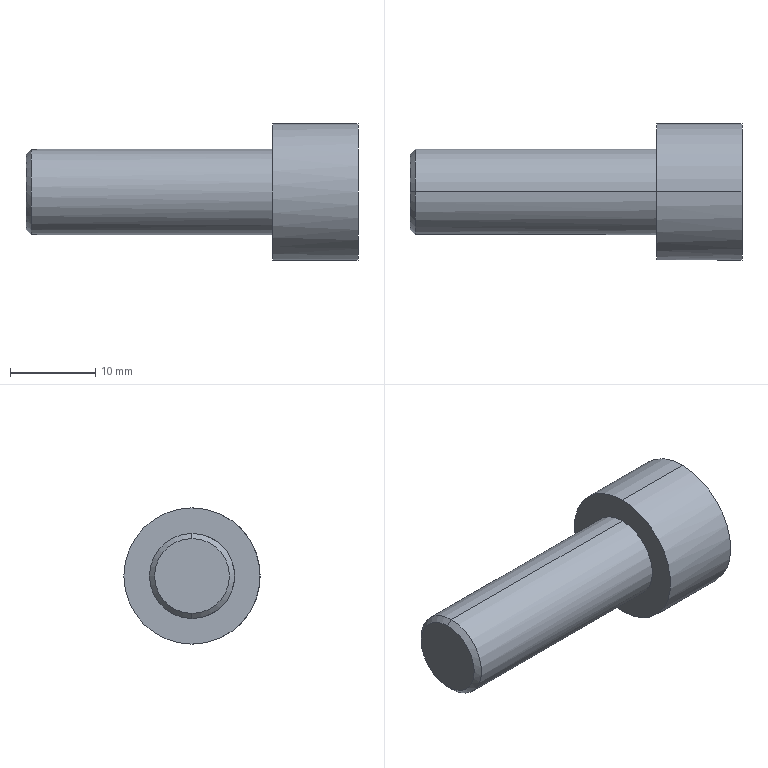Part | Creo | 1 solid | 16 faces | box 39 x 16 x 16 mm | volume 3917 mm3 | plane 10 | cylinder 4 | cone 2 | commonest cylinder face diameters 10 x2 16 x2
STEP:
#1=CARTESIAN_POINT('',(0.,0.,0.));
#2=DIRECTION('',(0.,0.,1.));
#3=DIRECTION('',(1.,0.,0.));
#4=AXIS2_PLACEMENT_3D('',#1,#2,#3);
#5=CARTESIAN_POINT('',(758.71,85.769,-129.619));
#6=VERTEX_POINT('',#5);
#7=CARTESIAN_POINT('',(758.71,90.769,-134.619));
#8=VERTEX_POINT('',#7);
#9=CARTESIAN_POINT('',(758.71,85.769,-134.619));
#10=DIRECTION('',(-1.,0.,0.));
#11=DIRECTION('',(0.,0.,1.));
#12=AXIS2_PLACEMENT_3D('',#9,#10,#11);
#13=CIRCLE('',#12,5.);
#14=EDGE_CURVE('',#6,#8,#13,.T.);
#15=ORIENTED_EDGE('',*,*,#14,.T.);
#16=CARTESIAN_POINT('',(758.71,85.769,-139.619));
#17=VERTEX_POINT('',#16);
#18=CARTESIAN_POINT('',(758.71,85.769,-134.619));
#19=DIRECTION('',(-1.,0.,0.));
#20=DIRECTION('',(0.,1.,0.));
#21=AXIS2_PLACEMENT_3D('',#18,#19,#20);
#22=CIRCLE('',#21,5.);
#23=EDGE_CURVE('',#8,#17,#22,.T.);
#24=ORIENTED_EDGE('',*,*,#23,.T.);
#25=CARTESIAN_POINT('',(787.101,85.769,-139.619));
#26=VERTEX_POINT('',#25);
#27=CARTESIAN_POINT('',(787.101,85.769,-139.619));
#28=DIRECTION('',(-1.,0.,0.));
#29=VECTOR('',#28,28.391);
#30=LINE('',#27,#29);
#31=EDGE_CURVE('',#26,#17,#30,.T.);
#32=ORIENTED_EDGE('',*,*,#31,.F.);
#33=CARTESIAN_POINT('',(787.101,90.769,-134.619));
#34=VERTEX_POINT('',#33);
#35=CARTESIAN_POINT('',(787.101,85.769,-134.619));
#36=DIRECTION('',(1.,0.,0.));
#37=DIRECTION('',(0.,0.,-1.));
#38=AXIS2_PLACEMENT_3D('',#35,#36,#37);
#39=CIRCLE('',#38,5.);
#40=EDGE_CURVE('',#26,#34,#39,.T.);
#41=ORIENTED_EDGE('',*,*,#40,.T.);
#42=CARTESIAN_POINT('',(787.101,85.769,-129.619));
#43=VERTEX_POINT('',#42);
#44=CARTESIAN_POINT('',(787.101,85.769,-134.619));
#45=DIRECTION('',(1.,0.,0.));
#46=DIRECTION('',(0.,1.,0.));
#47=AXIS2_PLACEMENT_3D('',#44,#45,#46);
#48=CIRCLE('',#47,5.);
#49=EDGE_CURVE('',#34,#43,#48,.T.);
#50=ORIENTED_EDGE('',*,*,#49,.T.);
#51=CARTESIAN_POINT('',(787.101,85.769,-129.619));
#52=DIRECTION('',(-1.,0.,0.));
#53=VECTOR('',#52,28.391);
#54=LINE('',#51,#53);
#55=EDGE_CURVE('',#43,#6,#54,.T.);
#56=ORIENTED_EDGE('',*,*,#55,.T.);
#57=EDGE_LOOP('',(#15,#24,#32,#41,#50,#56));
#58=FACE_OUTER_BOUND('',#57,.F.);
#59=CARTESIAN_POINT('',(787.101,85.769,-134.619));
#60=DIRECTION('',(-1.,0.,0.));
#61=DIRECTION('',(0.,0.,1.));
#62=AXIS2_PLACEMENT_3D('',#59,#60,#61);
#63=CYLINDRICAL_SURFACE('',#62,5.);
#64=ADVANCED_FACE('',(#58),#63,.T.);
#65=CARTESIAN_POINT('',(758.101,85.769,-130.228));
#66=VERTEX_POINT('',#65);
#67=CARTESIAN_POINT('',(758.101,90.16,-134.619));
#68=VERTEX_POINT('',#67);
#69=CARTESIAN_POINT('',(758.101,85.769,-134.619));
#70=DIRECTION('',(-1.,0.,0.));
#71=DIRECTION('',(0.,0.,1.));
#72=AXIS2_PLACEMENT_3D('',#69,#70,#71);
#73=CIRCLE('',#72,4.391);
#74=EDGE_CURVE('',#66,#68,#73,.T.);
#75=ORIENTED_EDGE('',*,*,#74,.T.);
#76=CARTESIAN_POINT('',(758.101,85.769,-139.01));
#77=VERTEX_POINT('',#76);
#78=CARTESIAN_POINT('',(758.101,85.769,-134.619));
#79=DIRECTION('',(-1.,0.,0.));
#80=DIRECTION('',(0.,1.,0.));
#81=AXIS2_PLACEMENT_3D('',#78,#79,#80);
#82=CIRCLE('',#81,4.391);
#83=EDGE_CURVE('',#68,#77,#82,.T.);
#84=ORIENTED_EDGE('',*,*,#83,.T.);
#85=CARTESIAN_POINT('',(758.101,85.769,-139.01));
#86=DIRECTION('',(0.7071,0.,-0.7071));
#87=VECTOR('',#86,0.8611);
#88=LINE('',#85,#87);
#89=EDGE_CURVE('',#77,#17,#88,.T.);
#90=ORIENTED_EDGE('',*,*,#89,.T.);
#91=ORIENTED_EDGE('',*,*,#23,.F.);
#92=ORIENTED_EDGE('',*,*,#14,.F.);
#93=CARTESIAN_POINT('',(758.101,85.769,-130.228));
#94=DIRECTION('',(0.7071,0.,0.7071));
#95=VECTOR('',#94,0.8611);
#96=LINE('',#93,#95);
#97=EDGE_CURVE('',#66,#6,#96,.T.);
#98=ORIENTED_EDGE('',*,*,#97,.F.);
#99=EDGE_LOOP('',(#75,#84,#90,#91,#92,#98));
#100=FACE_OUTER_BOUND('',#99,.F.);
#101=CARTESIAN_POINT('',(758.405,85.769,-134.619));
#102=DIRECTION('',(1.,0.,0.));
#103=DIRECTION('',(0.,0.,-1.));
#104=AXIS2_PLACEMENT_3D('',#101,#102,#103);
#105=CONICAL_SURFACE('',#104,4.696,45.);
#106=ADVANCED_FACE('',(#100),#105,.T.);
#107=ORIENTED_EDGE('',*,*,#83,.F.);
#108=ORIENTED_EDGE('',*,*,#74,.F.);
#109=CARTESIAN_POINT('',(758.101,81.378,-134.619));
#110=VERTEX_POINT('',#109);
#111=CARTESIAN_POINT('',(758.101,85.769,-134.619));
#112=DIRECTION('',(-1.,0.,0.));
#113=DIRECTION('',(0.,-1.,0.));
#114=AXIS2_PLACEMENT_3D('',#111,#112,#113);
#115=CIRCLE('',#114,4.391);
#116=EDGE_CURVE('',#110,#66,#115,.T.);
#117=ORIENTED_EDGE('',*,*,#116,.F.);
#118=CARTESIAN_POINT('',(758.101,85.769,-134.619));
#119=DIRECTION('',(-1.,0.,0.));
#120=DIRECTION('',(0.,0.,-1.));
#121=AXIS2_PLACEMENT_3D('',#118,#119,#120);
#122=CIRCLE('',#121,4.391);
#123=EDGE_CURVE('',#77,#110,#122,.T.);
#124=ORIENTED_EDGE('',*,*,#123,.F.);
#125=EDGE_LOOP('',(#107,#108,#117,#124));
#126=FACE_OUTER_BOUND('',#125,.F.);
#127=CARTESIAN_POINT('',(758.101,85.769,-134.619));
#128=DIRECTION('',(1.,0.,0.));
#129=DIRECTION('',(0.,0.,-1.));
#130=AXIS2_PLACEMENT_3D('',#127,#128,#129);
#131=PLANE('',#130);
#132=ADVANCED_FACE('',(#126),#131,.F.);
#133=ORIENTED_EDGE('',*,*,#116,.T.);
#134=ORIENTED_EDGE('',*,*,#97,.T.);
#135=CARTESIAN_POINT('',(758.71,85.769,-134.619));
#136=DIRECTION('',(-1.,0.,0.));
#137=DIRECTION('',(0.,0.,-1.));
#138=AXIS2_PLACEMENT_3D('',#135,#136,#137);
#139=CIRCLE('',#138,5.);
#140=EDGE_CURVE('',#17,#6,#139,.T.);
#141=ORIENTED_EDGE('',*,*,#140,.F.);
#142=ORIENTED_EDGE('',*,*,#89,.F.);
#143=ORIENTED_EDGE('',*,*,#123,.T.);
#144=EDGE_LOOP('',(#133,#134,#141,#142,#143));
#145=FACE_OUTER_BOUND('',#144,.F.);
#146=CARTESIAN_POINT('',(758.405,85.769,-134.619));
#147=DIRECTION('',(1.,0.,0.));
#148=DIRECTION('',(0.,0.,-1.));
#149=AXIS2_PLACEMENT_3D('',#146,#147,#148);
#150=CONICAL_SURFACE('',#149,4.696,45.);
#151=ADVANCED_FACE('',(#145),#150,.T.);
#152=ORIENTED_EDGE('',*,*,#140,.T.);
#153=ORIENTED_EDGE('',*,*,#55,.F.);
#154=CARTESIAN_POINT('',(787.101,80.769,-134.619));
#155=VERTEX_POINT('',#154);
#156=CARTESIAN_POINT('',(787.101,85.769,-134.619));
#157=DIRECTION('',(1.,0.,0.));
#158=DIRECTION('',(0.,0.,1.));
#159=AXIS2_PLACEMENT_3D('',#156,#157,#158);
#160=CIRCLE('',#159,5.);
#161=EDGE_CURVE('',#43,#155,#160,.T.);
#162=ORIENTED_EDGE('',*,*,#161,.T.);
#163=CARTESIAN_POINT('',(787.101,85.769,-134.619));
#164=DIRECTION('',(1.,0.,0.));
#165=DIRECTION('',(0.,-1.,0.));
#166=AXIS2_PLACEMENT_3D('',#163,#164,#165);
#167=CIRCLE('',#166,5.);
#168=EDGE_CURVE('',#155,#26,#167,.T.);
#169=ORIENTED_EDGE('',*,*,#168,.T.);
#170=ORIENTED_EDGE('',*,*,#31,.T.);
#171=EDGE_LOOP('',(#152,#153,#162,#169,#170));
#172=FACE_OUTER_BOUND('',#171,.F.);
#173=CARTESIAN_POINT('',(787.101,85.769,-134.619));
#174=DIRECTION('',(-1.,0.,0.));
#175=DIRECTION('',(0.,0.,1.));
#176=AXIS2_PLACEMENT_3D('',#173,#174,#175);
#177=CYLINDRICAL_SURFACE('',#176,5.);
#178=ADVANCED_FACE('',(#172),#177,.T.);
#179=CARTESIAN_POINT('',(787.101,93.769,-134.619));
#180=VERTEX_POINT('',#179);
#181=CARTESIAN_POINT('',(787.101,85.769,-142.619));
#182=VERTEX_POINT('',#181);
#183=CARTESIAN_POINT('',(787.101,85.769,-134.619));
#184=DIRECTION('',(-1.,0.,0.));
#185=DIRECTION('',(0.,1.,0.));
#186=AXIS2_PLACEMENT_3D('',#183,#184,#185);
#187=CIRCLE('',#186,8.);
#188=EDGE_CURVE('',#180,#182,#187,.T.);
#189=ORIENTED_EDGE('',*,*,#188,.F.);
#190=CARTESIAN_POINT('',(787.101,85.769,-126.619));
#191=VERTEX_POINT('',#190);
#192=CARTESIAN_POINT('',(787.101,85.769,-134.619));
#193=DIRECTION('',(-1.,0.,0.));
#194=DIRECTION('',(0.,0.,1.));
#195=AXIS2_PLACEMENT_3D('',#192,#193,#194);
#196=CIRCLE('',#195,8.);
#197=EDGE_CURVE('',#191,#180,#196,.T.);
#198=ORIENTED_EDGE('',*,*,#197,.F.);
#199=CARTESIAN_POINT('',(787.101,85.769,-134.619));
#200=DIRECTION('',(-1.,0.,0.));
#201=DIRECTION('',(0.,0.,-1.));
#202=AXIS2_PLACEMENT_3D('',#199,#200,#201);
#203=CIRCLE('',#202,8.);
#204=EDGE_CURVE('',#182,#191,#203,.T.);
#205=ORIENTED_EDGE('',*,*,#204,.F.);
#206=EDGE_LOOP('',(#189,#198,#205));
#207=FACE_OUTER_BOUND('',#206,.F.);
#208=ORIENTED_EDGE('',*,*,#49,.F.);
#209=ORIENTED_EDGE('',*,*,#40,.F.);
#210=ORIENTED_EDGE('',*,*,#168,.F.);
#211=ORIENTED_EDGE('',*,*,#161,.F.);
#212=EDGE_LOOP('',(#208,#209,#210,#211));
#213=FACE_BOUND('',#212,.F.);
#214=CARTESIAN_POINT('',(787.101,85.769,-134.619));
#215=DIRECTION('',(-1.,0.,0.));
#216=DIRECTION('',(0.,0.,1.));
#217=AXIS2_PLACEMENT_3D('',#214,#215,#216);
#218=PLANE('',#217);
#219=ADVANCED_FACE('',(#207,#213),#218,.T.);
#220=CARTESIAN_POINT('',(797.101,85.769,-142.619));
#221=VERTEX_POINT('',#220);
#222=CARTESIAN_POINT('',(797.101,93.769,-134.619));
#223=VERTEX_POINT('',#222);
#224=CARTESIAN_POINT('',(797.101,85.769,-134.619));
#225=DIRECTION('',(1.,0.,0.));
#226=DIRECTION('',(0.,0.,-1.));
#227=AXIS2_PLACEMENT_3D('',#224,#225,#226);
#228=CIRCLE('',#227,8.);
#229=EDGE_CURVE('',#221,#223,#228,.T.);
#230=ORIENTED_EDGE('',*,*,#229,.T.);
#231=CARTESIAN_POINT('',(797.101,85.769,-126.619));
#232=VERTEX_POINT('',#231);
#233=CARTESIAN_POINT('',(797.101,85.769,-134.619));
#234=DIRECTION('',(1.,0.,0.));
#235=DIRECTION('',(0.,1.,0.));
#236=AXIS2_PLACEMENT_3D('',#233,#234,#235);
#237=CIRCLE('',#236,8.);
#238=EDGE_CURVE('',#223,#232,#237,.T.);
#239=ORIENTED_EDGE('',*,*,#238,.T.);
#240=CARTESIAN_POINT('',(787.101,85.769,-126.619));
#241=DIRECTION('',(1.,0.,0.));
#242=VECTOR('',#241,10.);
#243=LINE('',#240,#242);
#244=EDGE_CURVE('',#191,#232,#243,.T.);
#245=ORIENTED_EDGE('',*,*,#244,.F.);
#246=ORIENTED_EDGE('',*,*,#197,.T.);
#247=ORIENTED_EDGE('',*,*,#188,.T.);
#248=CARTESIAN_POINT('',(787.101,85.769,-142.619));
#249=DIRECTION('',(1.,0.,0.));
#250=VECTOR('',#249,10.);
#251=LINE('',#248,#250);
#252=EDGE_CURVE('',#182,#221,#251,.T.);
#253=ORIENTED_EDGE('',*,*,#252,.T.);
#254=EDGE_LOOP('',(#230,#239,#245,#246,#247,#253));
#255=FACE_OUTER_BOUND('',#254,.F.);
#256=CARTESIAN_POINT('',(787.101,85.769,-134.619));
#257=DIRECTION('',(1.,0.,0.));
#258=DIRECTION('',(0.,0.,-1.));
#259=AXIS2_PLACEMENT_3D('',#256,#257,#258);
#260=CYLINDRICAL_SURFACE('',#259,8.);
#261=ADVANCED_FACE('',(#255),#260,.T.);
#262=ORIENTED_EDGE('',*,*,#238,.F.);
#263=ORIENTED_EDGE('',*,*,#229,.F.);
#264=CARTESIAN_POINT('',(797.101,77.769,-134.619));
#265=VERTEX_POINT('',#264);
#266=CARTESIAN_POINT('',(797.101,85.769,-134.619));
#267=DIRECTION('',(1.,0.,0.));
#268=DIRECTION('',(0.,-1.,0.));
#269=AXIS2_PLACEMENT_3D('',#266,#267,#268);
#270=CIRCLE('',#269,8.);
#271=EDGE_CURVE('',#265,#221,#270,.T.);
#272=ORIENTED_EDGE('',*,*,#271,.F.);
#273=CARTESIAN_POINT('',(797.101,85.769,-134.619));
#274=DIRECTION('',(1.,0.,0.));
#275=DIRECTION('',(0.,0.,1.));
#276=AXIS2_PLACEMENT_3D('',#273,#274,#275);
#277=CIRCLE('',#276,8.);
#278=EDGE_CURVE('',#232,#265,#277,.T.);
#279=ORIENTED_EDGE('',*,*,#278,.F.);
#280=EDGE_LOOP('',(#262,#263,#272,#279));
#281=FACE_OUTER_BOUND('',#280,.F.);
#282=CARTESIAN_POINT('',(797.101,88.078,-138.619));
#283=VERTEX_POINT('',#282);
#284=CARTESIAN_POINT('',(797.101,83.459,-138.619));
#285=VERTEX_POINT('',#284);
#286=CARTESIAN_POINT('',(797.101,88.078,-138.619));
#287=DIRECTION('',(0.,-1.,0.));
#288=VECTOR('',#287,4.619);
#289=LINE('',#286,#288);
#290=EDGE_CURVE('',#283,#285,#289,.T.);
#291=ORIENTED_EDGE('',*,*,#290,.F.);
#292=CARTESIAN_POINT('',(797.101,90.388,-134.619));
#293=VERTEX_POINT('',#292);
#294=CARTESIAN_POINT('',(797.101,90.388,-134.619));
#295=DIRECTION('',(0.,-0.5,-0.866));
#296=VECTOR('',#295,4.619);
#297=LINE('',#294,#296);
#298=EDGE_CURVE('',#293,#283,#297,.T.);
#299=ORIENTED_EDGE('',*,*,#298,.F.);
#300=CARTESIAN_POINT('',(797.101,88.078,-130.619));
#301=VERTEX_POINT('',#300);
#302=CARTESIAN_POINT('',(797.101,88.078,-130.619));
#303=DIRECTION('',(0.,0.5,-0.866));
#304=VECTOR('',#303,4.619);
#305=LINE('',#302,#304);
#306=EDGE_CURVE('',#301,#293,#305,.T.);
#307=ORIENTED_EDGE('',*,*,#306,.F.);
#308=CARTESIAN_POINT('',(797.101,83.459,-130.619));
#309=VERTEX_POINT('',#308);
#310=CARTESIAN_POINT('',(797.101,83.459,-130.619));
#311=DIRECTION('',(0.,1.,0.));
#312=VECTOR('',#311,4.619);
#313=LINE('',#310,#312);
#314=EDGE_CURVE('',#309,#301,#313,.T.);
#315=ORIENTED_EDGE('',*,*,#314,.F.);
#316=CARTESIAN_POINT('',(797.101,81.15,-134.619));
#317=VERTEX_POINT('',#316);
#318=CARTESIAN_POINT('',(797.101,81.15,-134.619));
#319=DIRECTION('',(0.,0.5,0.866));
#320=VECTOR('',#319,4.619);
#321=LINE('',#318,#320);
#322=EDGE_CURVE('',#317,#309,#321,.T.);
#323=ORIENTED_EDGE('',*,*,#322,.F.);
#324=CARTESIAN_POINT('',(797.101,83.459,-138.619));
#325=DIRECTION('',(0.,-0.5,0.866));
#326=VECTOR('',#325,4.619);
#327=LINE('',#324,#326);
#328=EDGE_CURVE('',#285,#317,#327,.T.);
#329=ORIENTED_EDGE('',*,*,#328,.F.);
#330=EDGE_LOOP('',(#291,#299,#307,#315,#323,#329));
#331=FACE_BOUND('',#330,.F.);
#332=CARTESIAN_POINT('',(797.101,85.769,-134.619));
#333=DIRECTION('',(1.,0.,0.));
#334=DIRECTION('',(0.,0.,-1.));
#335=AXIS2_PLACEMENT_3D('',#332,#333,#334);
#336=PLANE('',#335);
#337=ADVANCED_FACE('',(#281,#331),#336,.T.);
#338=ORIENTED_EDGE('',*,*,#290,.T.);
#339=CARTESIAN_POINT('',(790.501,83.459,-138.619));
#340=VERTEX_POINT('',#339);
#341=CARTESIAN_POINT('',(797.101,83.459,-138.619));
#342=DIRECTION('',(-1.,0.,0.));
#343=VECTOR('',#342,6.6);
#344=LINE('',#341,#343);
#345=EDGE_CURVE('',#285,#340,#344,.T.);
#346=ORIENTED_EDGE('',*,*,#345,.T.);
#347=CARTESIAN_POINT('',(790.501,88.078,-138.619));
#348=VERTEX_POINT('',#347);
#349=CARTESIAN_POINT('',(790.501,88.078,-138.619));
#350=DIRECTION('',(0.,-1.,0.));
#351=VECTOR('',#350,4.619);
#352=LINE('',#349,#351);
#353=EDGE_CURVE('',#348,#340,#352,.T.);
#354=ORIENTED_EDGE('',*,*,#353,.F.);
#355=CARTESIAN_POINT('',(797.101,88.078,-138.619));
#356=DIRECTION('',(-1.,0.,0.));
#357=VECTOR('',#356,6.6);
#358=LINE('',#355,#357);
#359=EDGE_CURVE('',#283,#348,#358,.T.);
#360=ORIENTED_EDGE('',*,*,#359,.F.);
#361=EDGE_LOOP('',(#338,#346,#354,#360));
#362=FACE_OUTER_BOUND('',#361,.F.);
#363=CARTESIAN_POINT('',(790.501,83.459,-138.619));
#364=DIRECTION('',(0.,0.,-1.));
#365=DIRECTION('',(-1.,0.,0.));
#366=AXIS2_PLACEMENT_3D('',#363,#364,#365);
#367=PLANE('',#366);
#368=ADVANCED_FACE('',(#362),#367,.F.);
#369=ORIENTED_EDGE('',*,*,#328,.T.);
#370=CARTESIAN_POINT('',(790.501,81.15,-134.619));
#371=VERTEX_POINT('',#370);
#372=CARTESIAN_POINT('',(797.101,81.15,-134.619));
#373=DIRECTION('',(-1.,0.,0.));
#374=VECTOR('',#373,6.6);
#375=LINE('',#372,#374);
#376=EDGE_CURVE('',#317,#371,#375,.T.);
#377=ORIENTED_EDGE('',*,*,#376,.T.);
#378=CARTESIAN_POINT('',(790.501,81.15,-134.619));
#379=DIRECTION('',(0.,0.5,-0.866));
#380=VECTOR('',#379,4.619);
#381=LINE('',#378,#380);
#382=EDGE_CURVE('',#371,#340,#381,.T.);
#383=ORIENTED_EDGE('',*,*,#382,.T.);
#384=ORIENTED_EDGE('',*,*,#345,.F.);
#385=EDGE_LOOP('',(#369,#377,#383,#384));
#386=FACE_OUTER_BOUND('',#385,.F.);
#387=CARTESIAN_POINT('',(790.501,81.15,-134.619));
#388=DIRECTION('',(0.,-0.866,-0.5));
#389=DIRECTION('',(0.,0.5,-0.866));
#390=AXIS2_PLACEMENT_3D('',#387,#388,#389);
#391=PLANE('',#390);
#392=ADVANCED_FACE('',(#386),#391,.F.);
#393=ORIENTED_EDGE('',*,*,#322,.T.);
#394=CARTESIAN_POINT('',(790.501,83.459,-130.619));
#395=VERTEX_POINT('',#394);
#396=CARTESIAN_POINT('',(797.101,83.459,-130.619));
#397=DIRECTION('',(-1.,0.,0.));
#398=VECTOR('',#397,6.6);
#399=LINE('',#396,#398);
#400=EDGE_CURVE('',#309,#395,#399,.T.);
#401=ORIENTED_EDGE('',*,*,#400,.T.);
#402=CARTESIAN_POINT('',(790.501,83.459,-130.619));
#403=DIRECTION('',(0.,-0.5,-0.866));
#404=VECTOR('',#403,4.619);
#405=LINE('',#402,#404);
#406=EDGE_CURVE('',#395,#371,#405,.T.);
#407=ORIENTED_EDGE('',*,*,#406,.T.);
#408=ORIENTED_EDGE('',*,*,#376,.F.);
#409=EDGE_LOOP('',(#393,#401,#407,#408));
#410=FACE_OUTER_BOUND('',#409,.F.);
#411=CARTESIAN_POINT('',(790.501,83.459,-130.619));
#412=DIRECTION('',(0.,-0.866,0.5));
#413=DIRECTION('',(0.,-0.5,-0.866));
#414=AXIS2_PLACEMENT_3D('',#411,#412,#413);
#415=PLANE('',#414);
#416=ADVANCED_FACE('',(#410),#415,.F.);
#417=ORIENTED_EDGE('',*,*,#314,.T.);
#418=CARTESIAN_POINT('',(790.501,88.078,-130.619));
#419=VERTEX_POINT('',#418);
#420=CARTESIAN_POINT('',(797.101,88.078,-130.619));
#421=DIRECTION('',(-1.,0.,0.));
#422=VECTOR('',#421,6.6);
#423=LINE('',#420,#422);
#424=EDGE_CURVE('',#301,#419,#423,.T.);
#425=ORIENTED_EDGE('',*,*,#424,.T.);
#426=CARTESIAN_POINT('',(790.501,83.459,-130.619));
#427=DIRECTION('',(0.,1.,0.));
#428=VECTOR('',#427,4.619);
#429=LINE('',#426,#428);
#430=EDGE_CURVE('',#395,#419,#429,.T.);
#431=ORIENTED_EDGE('',*,*,#430,.F.);
#432=ORIENTED_EDGE('',*,*,#400,.F.);
#433=EDGE_LOOP('',(#417,#425,#431,#432));
#434=FACE_OUTER_BOUND('',#433,.F.);
#435=CARTESIAN_POINT('',(790.501,88.078,-130.619));
#436=DIRECTION('',(0.,0.,1.));
#437=DIRECTION('',(1.,0.,0.));
#438=AXIS2_PLACEMENT_3D('',#435,#436,#437);
#439=PLANE('',#438);
#440=ADVANCED_FACE('',(#434),#439,.F.);
#441=ORIENTED_EDGE('',*,*,#306,.T.);
#442=CARTESIAN_POINT('',(790.501,90.388,-134.619));
#443=VERTEX_POINT('',#442);
#444=CARTESIAN_POINT('',(797.101,90.388,-134.619));
#445=DIRECTION('',(-1.,0.,0.));
#446=VECTOR('',#445,6.6);
#447=LINE('',#444,#446);
#448=EDGE_CURVE('',#293,#443,#447,.T.);
#449=ORIENTED_EDGE('',*,*,#448,.T.);
#450=CARTESIAN_POINT('',(790.501,90.388,-134.619));
#451=DIRECTION('',(0.,-0.5,0.866));
#452=VECTOR('',#451,4.619);
#453=LINE('',#450,#452);
#454=EDGE_CURVE('',#443,#419,#453,.T.);
#455=ORIENTED_EDGE('',*,*,#454,.T.);
#456=ORIENTED_EDGE('',*,*,#424,.F.);
#457=EDGE_LOOP('',(#441,#449,#455,#456));
#458=FACE_OUTER_BOUND('',#457,.F.);
#459=CARTESIAN_POINT('',(790.501,90.388,-134.619));
#460=DIRECTION('',(0.,0.866,0.5));
#461=DIRECTION('',(0.,-0.5,0.866));
#462=AXIS2_PLACEMENT_3D('',#459,#460,#461);
#463=PLANE('',#462);
#464=ADVANCED_FACE('',(#458),#463,.F.);
#465=ORIENTED_EDGE('',*,*,#298,.T.);
#466=ORIENTED_EDGE('',*,*,#359,.T.);
#467=CARTESIAN_POINT('',(790.501,88.078,-138.619));
#468=DIRECTION('',(0.,0.5,0.866));
#469=VECTOR('',#468,4.619);
#470=LINE('',#467,#469);
#471=EDGE_CURVE('',#348,#443,#470,.T.);
#472=ORIENTED_EDGE('',*,*,#471,.T.);
#473=ORIENTED_EDGE('',*,*,#448,.F.);
#474=EDGE_LOOP('',(#465,#466,#472,#473));
#475=FACE_OUTER_BOUND('',#474,.F.);
#476=CARTESIAN_POINT('',(790.501,88.078,-138.619));
#477=DIRECTION('',(0.,0.866,-0.5));
#478=DIRECTION('',(0.,0.5,0.866));
#479=AXIS2_PLACEMENT_3D('',#476,#477,#478);
#480=PLANE('',#479);
#481=ADVANCED_FACE('',(#475),#480,.F.);
#482=ORIENTED_EDGE('',*,*,#353,.T.);
#483=ORIENTED_EDGE('',*,*,#382,.F.);
#484=ORIENTED_EDGE('',*,*,#406,.F.);
#485=ORIENTED_EDGE('',*,*,#430,.T.);
#486=ORIENTED_EDGE('',*,*,#454,.F.);
#487=ORIENTED_EDGE('',*,*,#471,.F.);
#488=EDGE_LOOP('',(#482,#483,#484,#485,#486,#487));
#489=FACE_OUTER_BOUND('',#488,.F.);
#490=CARTESIAN_POINT('',(790.501,88.078,-138.619));
#491=DIRECTION('',(1.,0.,0.));
#492=DIRECTION('',(0.,0.,-1.));
#493=AXIS2_PLACEMENT_3D('',#490,#491,#492);
#494=PLANE('',#493);
#495=ADVANCED_FACE('',(#489),#494,.T.);
#496=ORIENTED_EDGE('',*,*,#271,.T.);
#497=ORIENTED_EDGE('',*,*,#252,.F.);
#498=ORIENTED_EDGE('',*,*,#204,.T.);
#499=ORIENTED_EDGE('',*,*,#244,.T.);
#500=ORIENTED_EDGE('',*,*,#278,.T.);
#501=EDGE_LOOP('',(#496,#497,#498,#499,#500));
#502=FACE_OUTER_BOUND('',#501,.F.);
#503=CARTESIAN_POINT('',(787.101,85.769,-134.619));
#504=DIRECTION('',(1.,0.,0.));
#505=DIRECTION('',(0.,0.,-1.));
#506=AXIS2_PLACEMENT_3D('',#503,#504,#505);
#507=CYLINDRICAL_SURFACE('',#506,8.);
#508=ADVANCED_FACE('',(#502),#507,.T.);
#509=CLOSED_SHELL('',(#64,#106,#132,#151,#178,#219,#261,#337,#368,#392,#416,#440,#464,#481,#495,#508));
#510=MANIFOLD_SOLID_BREP('',#509);
#511=(LENGTH_UNIT()NAMED_UNIT(*)SI_UNIT(.MILLI.,.METRE.));
#512=UNCERTAINTY_MEASURE_WITH_UNIT(LENGTH_MEASURE(0.004509),#511,'','');
#513=(NAMED_UNIT(*)PLANE_ANGLE_UNIT()SI_UNIT($,.RADIAN.));
#514=PLANE_ANGLE_MEASURE_WITH_UNIT(PLANE_ANGLE_MEASURE(0.01745),#513);
#515=(CONVERSION_BASED_UNIT('DEGREE',#514)NAMED_UNIT(*)PLANE_ANGLE_UNIT());
#516=(NAMED_UNIT(*)SI_UNIT($,.STERADIAN.)SOLID_ANGLE_UNIT());
#517=(GEOMETRIC_REPRESENTATION_CONTEXT(3)GLOBAL_UNCERTAINTY_ASSIGNED_CONTEXT((#512))GLOBAL_UNIT_ASSIGNED_CONTEXT((#511,#515,#516))REPRESENTATION_CONTEXT('',''));
#518=ADVANCED_BREP_SHAPE_REPRESENTATION('',(#4,#510),#517);